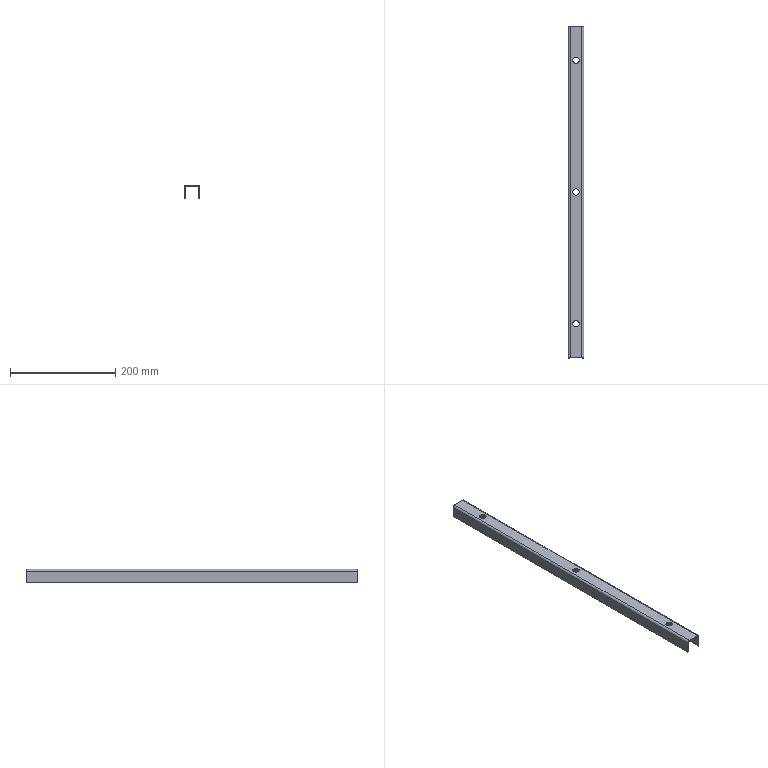Part | SolidWorks | features EdgeFlange 1, FlatPattern 1, ICE 1, SMBaseFlange 1, SheetMetal 1 | 1 solid | 28 faces | box 30 x 630 x 25 mm | volume 91837 mm3 | plane 18 | cylinder 10 | commonest cylinder face diameters 12 x6 4 x2 8 x2
STEP:
#1=CARTESIAN_POINT('',(6.,250.,-2.));
#2=VERTEX_POINT('',#1);
#3=CARTESIAN_POINT('',(-6.,250.,-2.));
#4=VERTEX_POINT('',#3);
#5=CARTESIAN_POINT('',(0.,250.,-2.));
#6=DIRECTION('',(0.,0.,-1.));
#7=DIRECTION('',(-1.,0.,0.));
#8=AXIS2_PLACEMENT_3D('',#5,#6,#7);
#9=CIRCLE('',#8,6.);
#10=EDGE_CURVE('',#2,#4,#9,.T.);
#11=ORIENTED_EDGE('',*,*,#10,.T.);
#12=CARTESIAN_POINT('',(-6.,250.,0.));
#13=VERTEX_POINT('',#12);
#14=CARTESIAN_POINT('',(-6.,250.,-25.));
#15=DIRECTION('',(0.,0.,1.));
#16=VECTOR('',#15,1000.);
#17=LINE('',#14,#16);
#18=EDGE_CURVE('',#4,#13,#17,.T.);
#19=ORIENTED_EDGE('',*,*,#18,.T.);
#20=CARTESIAN_POINT('',(6.,250.,0.));
#21=VERTEX_POINT('',#20);
#22=CARTESIAN_POINT('',(0.,250.,0.));
#23=DIRECTION('',(0.,0.,1.));
#24=DIRECTION('',(1.,0.,0.));
#25=AXIS2_PLACEMENT_3D('',#22,#23,#24);
#26=CIRCLE('',#25,6.);
#27=EDGE_CURVE('',#13,#21,#26,.T.);
#28=ORIENTED_EDGE('',*,*,#27,.T.);
#29=CARTESIAN_POINT('',(6.,250.,-25.));
#30=DIRECTION('',(0.,0.,1.));
#31=VECTOR('',#30,1000.);
#32=LINE('',#29,#31);
#33=EDGE_CURVE('',#2,#21,#32,.T.);
#34=ORIENTED_EDGE('',*,*,#33,.F.);
#35=EDGE_LOOP('',(#11,#19,#28,#34));
#36=FACE_OUTER_BOUND('',#35,.T.);
#37=CARTESIAN_POINT('',(0.,250.,-25.));
#38=DIRECTION('',(0.,0.,1.));
#39=DIRECTION('',(1.,0.,0.));
#40=AXIS2_PLACEMENT_3D('',#37,#38,#39);
#41=CYLINDRICAL_SURFACE('',#40,6.);
#42=ADVANCED_FACE('',(#36),#41,.F.);
#43=CARTESIAN_POINT('',(6.,-250.,-2.));
#44=VERTEX_POINT('',#43);
#45=CARTESIAN_POINT('',(-6.,-250.,-2.));
#46=VERTEX_POINT('',#45);
#47=CARTESIAN_POINT('',(0.,-250.,-2.));
#48=DIRECTION('',(0.,0.,-1.));
#49=DIRECTION('',(-1.,0.,0.));
#50=AXIS2_PLACEMENT_3D('',#47,#48,#49);
#51=CIRCLE('',#50,6.);
#52=EDGE_CURVE('',#44,#46,#51,.T.);
#53=ORIENTED_EDGE('',*,*,#52,.T.);
#54=CARTESIAN_POINT('',(-6.,-250.,0.));
#55=VERTEX_POINT('',#54);
#56=CARTESIAN_POINT('',(-6.,-250.,-25.));
#57=DIRECTION('',(0.,0.,1.));
#58=VECTOR('',#57,1000.);
#59=LINE('',#56,#58);
#60=EDGE_CURVE('',#46,#55,#59,.T.);
#61=ORIENTED_EDGE('',*,*,#60,.T.);
#62=CARTESIAN_POINT('',(6.,-250.,0.));
#63=VERTEX_POINT('',#62);
#64=CARTESIAN_POINT('',(0.,-250.,0.));
#65=DIRECTION('',(0.,0.,1.));
#66=DIRECTION('',(1.,0.,0.));
#67=AXIS2_PLACEMENT_3D('',#64,#65,#66);
#68=CIRCLE('',#67,6.);
#69=EDGE_CURVE('',#55,#63,#68,.T.);
#70=ORIENTED_EDGE('',*,*,#69,.T.);
#71=CARTESIAN_POINT('',(6.,-250.,-25.));
#72=DIRECTION('',(0.,0.,1.));
#73=VECTOR('',#72,1000.);
#74=LINE('',#71,#73);
#75=EDGE_CURVE('',#44,#63,#74,.T.);
#76=ORIENTED_EDGE('',*,*,#75,.F.);
#77=EDGE_LOOP('',(#53,#61,#70,#76));
#78=FACE_OUTER_BOUND('',#77,.T.);
#79=CARTESIAN_POINT('',(0.,-250.,-25.));
#80=DIRECTION('',(0.,0.,1.));
#81=DIRECTION('',(1.,0.,0.));
#82=AXIS2_PLACEMENT_3D('',#79,#80,#81);
#83=CYLINDRICAL_SURFACE('',#82,6.);
#84=ADVANCED_FACE('',(#78),#83,.F.);
#85=CARTESIAN_POINT('',(6.,0.,-2.));
#86=VERTEX_POINT('',#85);
#87=CARTESIAN_POINT('',(-6.,0.,-2.));
#88=VERTEX_POINT('',#87);
#89=CARTESIAN_POINT('',(0.,0.,-2.));
#90=DIRECTION('',(0.,0.,-1.));
#91=DIRECTION('',(-1.,0.,0.));
#92=AXIS2_PLACEMENT_3D('',#89,#90,#91);
#93=CIRCLE('',#92,6.);
#94=EDGE_CURVE('',#86,#88,#93,.T.);
#95=ORIENTED_EDGE('',*,*,#94,.T.);
#96=CARTESIAN_POINT('',(-6.,0.,0.));
#97=VERTEX_POINT('',#96);
#98=CARTESIAN_POINT('',(-6.,0.,-25.));
#99=DIRECTION('',(0.,0.,1.));
#100=VECTOR('',#99,1000.);
#101=LINE('',#98,#100);
#102=EDGE_CURVE('',#88,#97,#101,.T.);
#103=ORIENTED_EDGE('',*,*,#102,.T.);
#104=CARTESIAN_POINT('',(6.,0.,0.));
#105=VERTEX_POINT('',#104);
#106=CARTESIAN_POINT('',(0.,0.,0.));
#107=DIRECTION('',(0.,0.,1.));
#108=DIRECTION('',(1.,0.,0.));
#109=AXIS2_PLACEMENT_3D('',#106,#107,#108);
#110=CIRCLE('',#109,6.);
#111=EDGE_CURVE('',#97,#105,#110,.T.);
#112=ORIENTED_EDGE('',*,*,#111,.T.);
#113=CARTESIAN_POINT('',(6.,0.,-25.));
#114=DIRECTION('',(0.,0.,1.));
#115=VECTOR('',#114,1000.);
#116=LINE('',#113,#115);
#117=EDGE_CURVE('',#86,#105,#116,.T.);
#118=ORIENTED_EDGE('',*,*,#117,.F.);
#119=EDGE_LOOP('',(#95,#103,#112,#118));
#120=FACE_OUTER_BOUND('',#119,.T.);
#121=CARTESIAN_POINT('',(0.,0.,-25.));
#122=DIRECTION('',(0.,0.,1.));
#123=DIRECTION('',(1.,0.,0.));
#124=AXIS2_PLACEMENT_3D('',#121,#122,#123);
#125=CYLINDRICAL_SURFACE('',#124,6.);
#126=ADVANCED_FACE('',(#120),#125,.F.);
#127=ORIENTED_EDGE('',*,*,#10,.F.);
#128=CARTESIAN_POINT('',(0.,250.,-2.));
#129=DIRECTION('',(0.,0.,-1.));
#130=DIRECTION('',(-1.,0.,0.));
#131=AXIS2_PLACEMENT_3D('',#128,#129,#130);
#132=CIRCLE('',#131,6.);
#133=EDGE_CURVE('',#4,#2,#132,.T.);
#134=ORIENTED_EDGE('',*,*,#133,.F.);
#135=EDGE_LOOP('',(#127,#134));
#136=FACE_BOUND('',#135,.T.);
#137=ORIENTED_EDGE('',*,*,#52,.F.);
#138=CARTESIAN_POINT('',(0.,-250.,-2.));
#139=DIRECTION('',(0.,0.,-1.));
#140=DIRECTION('',(-1.,0.,0.));
#141=AXIS2_PLACEMENT_3D('',#138,#139,#140);
#142=CIRCLE('',#141,6.);
#143=EDGE_CURVE('',#46,#44,#142,.T.);
#144=ORIENTED_EDGE('',*,*,#143,.F.);
#145=EDGE_LOOP('',(#137,#144));
#146=FACE_BOUND('',#145,.T.);
#147=ORIENTED_EDGE('',*,*,#94,.F.);
#148=CARTESIAN_POINT('',(0.,0.,-2.));
#149=DIRECTION('',(0.,0.,-1.));
#150=DIRECTION('',(-1.,0.,0.));
#151=AXIS2_PLACEMENT_3D('',#148,#149,#150);
#152=CIRCLE('',#151,6.);
#153=EDGE_CURVE('',#88,#86,#152,.T.);
#154=ORIENTED_EDGE('',*,*,#153,.F.);
#155=EDGE_LOOP('',(#147,#154));
#156=FACE_BOUND('',#155,.T.);
#157=CARTESIAN_POINT('',(-11.,-315.,-2.));
#158=VERTEX_POINT('',#157);
#159=CARTESIAN_POINT('',(11.,-315.,-2.));
#160=VERTEX_POINT('',#159);
#161=CARTESIAN_POINT('',(-15.,-315.,-2.));
#162=DIRECTION('',(1.,0.,0.));
#163=VECTOR('',#162,1000.);
#164=LINE('',#161,#163);
#165=EDGE_CURVE('',#158,#160,#164,.T.);
#166=ORIENTED_EDGE('',*,*,#165,.F.);
#167=CARTESIAN_POINT('',(-11.,315.,-2.));
#168=VERTEX_POINT('',#167);
#169=CARTESIAN_POINT('',(-11.,315.,-2.));
#170=DIRECTION('',(0.,-1.,0.));
#171=VECTOR('',#170,1000.);
#172=LINE('',#169,#171);
#173=EDGE_CURVE('',#168,#158,#172,.T.);
#174=ORIENTED_EDGE('',*,*,#173,.F.);
#175=CARTESIAN_POINT('',(11.,315.,-2.));
#176=VERTEX_POINT('',#175);
#177=CARTESIAN_POINT('',(-15.,315.,-2.));
#178=DIRECTION('',(-1.,0.,0.));
#179=VECTOR('',#178,1000.);
#180=LINE('',#177,#179);
#181=EDGE_CURVE('',#176,#168,#180,.T.);
#182=ORIENTED_EDGE('',*,*,#181,.F.);
#183=CARTESIAN_POINT('',(11.,-315.,-2.));
#184=DIRECTION('',(0.,1.,0.));
#185=VECTOR('',#184,1000.);
#186=LINE('',#183,#185);
#187=EDGE_CURVE('',#160,#176,#186,.T.);
#188=ORIENTED_EDGE('',*,*,#187,.F.);
#189=EDGE_LOOP('',(#166,#174,#182,#188));
#190=FACE_OUTER_BOUND('',#189,.T.);
#191=CARTESIAN_POINT('',(0.,0.,-2.));
#192=DIRECTION('',(0.,0.,-1.));
#193=DIRECTION('',(-1.,0.,0.));
#194=AXIS2_PLACEMENT_3D('',#191,#192,#193);
#195=PLANE('',#194);
#196=ADVANCED_FACE('',(#136,#146,#156,#190),#195,.T.);
#197=CARTESIAN_POINT('',(0.,250.,0.));
#198=DIRECTION('',(0.,0.,1.));
#199=DIRECTION('',(1.,0.,0.));
#200=AXIS2_PLACEMENT_3D('',#197,#198,#199);
#201=CIRCLE('',#200,6.);
#202=EDGE_CURVE('',#21,#13,#201,.T.);
#203=ORIENTED_EDGE('',*,*,#202,.F.);
#204=ORIENTED_EDGE('',*,*,#27,.F.);
#205=EDGE_LOOP('',(#203,#204));
#206=FACE_BOUND('',#205,.T.);
#207=CARTESIAN_POINT('',(0.,-250.,0.));
#208=DIRECTION('',(0.,0.,1.));
#209=DIRECTION('',(1.,0.,0.));
#210=AXIS2_PLACEMENT_3D('',#207,#208,#209);
#211=CIRCLE('',#210,6.);
#212=EDGE_CURVE('',#63,#55,#211,.T.);
#213=ORIENTED_EDGE('',*,*,#212,.F.);
#214=ORIENTED_EDGE('',*,*,#69,.F.);
#215=EDGE_LOOP('',(#213,#214));
#216=FACE_BOUND('',#215,.T.);
#217=CARTESIAN_POINT('',(0.,0.,0.));
#218=DIRECTION('',(0.,0.,1.));
#219=DIRECTION('',(1.,0.,0.));
#220=AXIS2_PLACEMENT_3D('',#217,#218,#219);
#221=CIRCLE('',#220,6.);
#222=EDGE_CURVE('',#105,#97,#221,.T.);
#223=ORIENTED_EDGE('',*,*,#222,.F.);
#224=ORIENTED_EDGE('',*,*,#111,.F.);
#225=EDGE_LOOP('',(#223,#224));
#226=FACE_BOUND('',#225,.T.);
#227=CARTESIAN_POINT('',(-11.,315.,0.));
#228=VERTEX_POINT('',#227);
#229=CARTESIAN_POINT('',(-11.,-315.,0.));
#230=VERTEX_POINT('',#229);
#231=CARTESIAN_POINT('',(-11.,315.,0.));
#232=DIRECTION('',(0.,-1.,0.));
#233=VECTOR('',#232,1000.);
#234=LINE('',#231,#233);
#235=EDGE_CURVE('',#228,#230,#234,.T.);
#236=ORIENTED_EDGE('',*,*,#235,.T.);
#237=CARTESIAN_POINT('',(11.,-315.,0.));
#238=VERTEX_POINT('',#237);
#239=CARTESIAN_POINT('',(-15.,-315.,0.));
#240=DIRECTION('',(1.,0.,0.));
#241=VECTOR('',#240,1000.);
#242=LINE('',#239,#241);
#243=EDGE_CURVE('',#230,#238,#242,.T.);
#244=ORIENTED_EDGE('',*,*,#243,.T.);
#245=CARTESIAN_POINT('',(11.,315.,0.));
#246=VERTEX_POINT('',#245);
#247=CARTESIAN_POINT('',(11.,-315.,0.));
#248=DIRECTION('',(0.,1.,0.));
#249=VECTOR('',#248,1000.);
#250=LINE('',#247,#249);
#251=EDGE_CURVE('',#238,#246,#250,.T.);
#252=ORIENTED_EDGE('',*,*,#251,.T.);
#253=CARTESIAN_POINT('',(-15.,315.,0.));
#254=DIRECTION('',(-1.,0.,0.));
#255=VECTOR('',#254,1000.);
#256=LINE('',#253,#255);
#257=EDGE_CURVE('',#246,#228,#256,.T.);
#258=ORIENTED_EDGE('',*,*,#257,.T.);
#259=EDGE_LOOP('',(#236,#244,#252,#258));
#260=FACE_OUTER_BOUND('',#259,.T.);
#261=CARTESIAN_POINT('',(0.,0.,0.));
#262=DIRECTION('',(0.,0.,-1.));
#263=DIRECTION('',(-1.,0.,0.));
#264=AXIS2_PLACEMENT_3D('',#261,#262,#263);
#265=PLANE('',#264);
#266=ADVANCED_FACE('',(#206,#216,#226,#260),#265,.F.);
#267=ORIENTED_EDGE('',*,*,#181,.T.);
#268=CARTESIAN_POINT('',(-11.,315.,-2.));
#269=DIRECTION('',(0.,0.,1.));
#270=VECTOR('',#269,1000.);
#271=LINE('',#268,#270);
#272=EDGE_CURVE('',#168,#228,#271,.T.);
#273=ORIENTED_EDGE('',*,*,#272,.T.);
#274=ORIENTED_EDGE('',*,*,#257,.F.);
#275=CARTESIAN_POINT('',(11.,315.,-2.));
#276=DIRECTION('',(0.,0.,1.));
#277=VECTOR('',#276,1000.);
#278=LINE('',#275,#277);
#279=EDGE_CURVE('',#176,#246,#278,.T.);
#280=ORIENTED_EDGE('',*,*,#279,.F.);
#281=EDGE_LOOP('',(#267,#273,#274,#280));
#282=FACE_OUTER_BOUND('',#281,.T.);
#283=CARTESIAN_POINT('',(-15.,315.,-2.));
#284=DIRECTION('',(0.,1.,0.));
#285=DIRECTION('',(0.,0.,1.));
#286=AXIS2_PLACEMENT_3D('',#283,#284,#285);
#287=PLANE('',#286);
#288=ADVANCED_FACE('',(#282),#287,.T.);
#289=CARTESIAN_POINT('',(-11.,-315.,-2.));
#290=DIRECTION('',(0.,0.,1.));
#291=VECTOR('',#290,1000.);
#292=LINE('',#289,#291);
#293=EDGE_CURVE('',#158,#230,#292,.T.);
#294=ORIENTED_EDGE('',*,*,#293,.F.);
#295=ORIENTED_EDGE('',*,*,#165,.T.);
#296=CARTESIAN_POINT('',(11.,-315.,-2.));
#297=DIRECTION('',(0.,0.,1.));
#298=VECTOR('',#297,1000.);
#299=LINE('',#296,#298);
#300=EDGE_CURVE('',#160,#238,#299,.T.);
#301=ORIENTED_EDGE('',*,*,#300,.T.);
#302=ORIENTED_EDGE('',*,*,#243,.F.);
#303=EDGE_LOOP('',(#294,#295,#301,#302));
#304=FACE_OUTER_BOUND('',#303,.T.);
#305=CARTESIAN_POINT('',(-15.,-315.,-2.));
#306=DIRECTION('',(0.,-1.,0.));
#307=DIRECTION('',(0.,0.,-1.));
#308=AXIS2_PLACEMENT_3D('',#305,#306,#307);
#309=PLANE('',#308);
#310=ADVANCED_FACE('',(#304),#309,.T.);
#311=CARTESIAN_POINT('',(13.,315.,-4.));
#312=VERTEX_POINT('',#311);
#313=CARTESIAN_POINT('',(15.,315.,-4.));
#314=VERTEX_POINT('',#313);
#315=CARTESIAN_POINT('',(15.,315.,-4.));
#316=DIRECTION('',(1.,0.,0.));
#317=VECTOR('',#316,1000.);
#318=LINE('',#315,#317);
#319=EDGE_CURVE('',#312,#314,#318,.T.);
#320=ORIENTED_EDGE('',*,*,#319,.F.);
#321=CARTESIAN_POINT('',(11.,315.,-4.));
#322=DIRECTION('',(0.,1.,0.));
#323=DIRECTION('',(0.,0.,-1.));
#324=AXIS2_PLACEMENT_3D('',#321,#322,#323);
#325=CIRCLE('',#324,2.);
#326=EDGE_CURVE('',#176,#312,#325,.T.);
#327=ORIENTED_EDGE('',*,*,#326,.F.);
#328=ORIENTED_EDGE('',*,*,#279,.T.);
#329=CARTESIAN_POINT('',(11.,315.,-4.));
#330=DIRECTION('',(0.,1.,0.));
#331=DIRECTION('',(0.,0.,-1.));
#332=AXIS2_PLACEMENT_3D('',#329,#330,#331);
#333=CIRCLE('',#332,4.);
#334=EDGE_CURVE('',#246,#314,#333,.T.);
#335=ORIENTED_EDGE('',*,*,#334,.T.);
#336=EDGE_LOOP('',(#320,#327,#328,#335));
#337=FACE_OUTER_BOUND('',#336,.T.);
#338=CARTESIAN_POINT('',(11.,315.,-4.));
#339=DIRECTION('',(0.,1.,0.));
#340=DIRECTION('',(0.,0.,1.));
#341=AXIS2_PLACEMENT_3D('',#338,#339,#340);
#342=PLANE('',#341);
#343=ADVANCED_FACE('',(#337),#342,.T.);
#344=CARTESIAN_POINT('',(13.,-315.,-4.));
#345=VERTEX_POINT('',#344);
#346=CARTESIAN_POINT('',(11.,-315.,-4.));
#347=DIRECTION('',(0.,-1.,0.));
#348=DIRECTION('',(0.,0.,-1.));
#349=AXIS2_PLACEMENT_3D('',#346,#347,#348);
#350=CIRCLE('',#349,2.);
#351=EDGE_CURVE('',#345,#160,#350,.T.);
#352=ORIENTED_EDGE('',*,*,#351,.F.);
#353=CARTESIAN_POINT('',(15.,-315.,-4.));
#354=VERTEX_POINT('',#353);
#355=CARTESIAN_POINT('',(13.,-315.,-4.));
#356=DIRECTION('',(1.,0.,0.));
#357=VECTOR('',#356,1000.);
#358=LINE('',#355,#357);
#359=EDGE_CURVE('',#345,#354,#358,.T.);
#360=ORIENTED_EDGE('',*,*,#359,.T.);
#361=CARTESIAN_POINT('',(11.,-315.,-4.));
#362=DIRECTION('',(0.,-1.,0.));
#363=DIRECTION('',(0.,0.,-1.));
#364=AXIS2_PLACEMENT_3D('',#361,#362,#363);
#365=CIRCLE('',#364,4.);
#366=EDGE_CURVE('',#354,#238,#365,.T.);
#367=ORIENTED_EDGE('',*,*,#366,.T.);
#368=ORIENTED_EDGE('',*,*,#300,.F.);
#369=EDGE_LOOP('',(#352,#360,#367,#368));
#370=FACE_OUTER_BOUND('',#369,.T.);
#371=CARTESIAN_POINT('',(11.,-315.,-4.));
#372=DIRECTION('',(0.,1.,0.));
#373=DIRECTION('',(0.,0.,1.));
#374=AXIS2_PLACEMENT_3D('',#371,#372,#373);
#375=PLANE('',#374);
#376=ADVANCED_FACE('',(#370),#375,.F.);
#377=ORIENTED_EDGE('',*,*,#251,.F.);
#378=ORIENTED_EDGE('',*,*,#366,.F.);
#379=CARTESIAN_POINT('',(15.,0.,-4.));
#380=DIRECTION('',(0.,-1.,0.));
#381=VECTOR('',#380,1000.);
#382=LINE('',#379,#381);
#383=EDGE_CURVE('',#314,#354,#382,.T.);
#384=ORIENTED_EDGE('',*,*,#383,.F.);
#385=ORIENTED_EDGE('',*,*,#334,.F.);
#386=EDGE_LOOP('',(#377,#378,#384,#385));
#387=FACE_OUTER_BOUND('',#386,.T.);
#388=CARTESIAN_POINT('',(11.,-315.,-4.));
#389=DIRECTION('',(0.,-1.,0.));
#390=DIRECTION('',(1.,0.,0.));
#391=AXIS2_PLACEMENT_3D('',#388,#389,#390);
#392=CYLINDRICAL_SURFACE('',#391,4.);
#393=ADVANCED_FACE('',(#387),#392,.T.);
#394=ORIENTED_EDGE('',*,*,#187,.T.);
#395=ORIENTED_EDGE('',*,*,#326,.T.);
#396=CARTESIAN_POINT('',(13.,315.,-4.));
#397=DIRECTION('',(0.,-1.,0.));
#398=VECTOR('',#397,1000.);
#399=LINE('',#396,#398);
#400=EDGE_CURVE('',#312,#345,#399,.T.);
#401=ORIENTED_EDGE('',*,*,#400,.T.);
#402=ORIENTED_EDGE('',*,*,#351,.T.);
#403=EDGE_LOOP('',(#394,#395,#401,#402));
#404=FACE_OUTER_BOUND('',#403,.T.);
#405=CARTESIAN_POINT('',(11.,-315.,-4.));
#406=DIRECTION('',(0.,-1.,0.));
#407=DIRECTION('',(1.,0.,0.));
#408=AXIS2_PLACEMENT_3D('',#405,#406,#407);
#409=CYLINDRICAL_SURFACE('',#408,2.);
#410=ADVANCED_FACE('',(#404),#409,.F.);
#411=CARTESIAN_POINT('',(15.,-315.,-25.));
#412=VERTEX_POINT('',#411);
#413=CARTESIAN_POINT('',(15.,-315.,-2.));
#414=DIRECTION('',(0.,0.,1.));
#415=VECTOR('',#414,1000.);
#416=LINE('',#413,#415);
#417=EDGE_CURVE('',#412,#354,#416,.T.);
#418=ORIENTED_EDGE('',*,*,#417,.T.);
#419=ORIENTED_EDGE('',*,*,#359,.F.);
#420=CARTESIAN_POINT('',(13.,-315.,-25.));
#421=VERTEX_POINT('',#420);
#422=CARTESIAN_POINT('',(13.,-315.,0.));
#423=DIRECTION('',(0.,0.,1.));
#424=VECTOR('',#423,1000.);
#425=LINE('',#422,#424);
#426=EDGE_CURVE('',#421,#345,#425,.T.);
#427=ORIENTED_EDGE('',*,*,#426,.F.);
#428=CARTESIAN_POINT('',(15.,-315.,-25.));
#429=DIRECTION('',(-1.,0.,0.));
#430=VECTOR('',#429,1000.);
#431=LINE('',#428,#430);
#432=EDGE_CURVE('',#412,#421,#431,.T.);
#433=ORIENTED_EDGE('',*,*,#432,.F.);
#434=EDGE_LOOP('',(#418,#419,#427,#433));
#435=FACE_OUTER_BOUND('',#434,.T.);
#436=CARTESIAN_POINT('',(15.,-315.,-2.));
#437=DIRECTION('',(0.,-1.,0.));
#438=DIRECTION('',(0.,0.,-1.));
#439=AXIS2_PLACEMENT_3D('',#436,#437,#438);
#440=PLANE('',#439);
#441=ADVANCED_FACE('',(#435),#440,.T.);
#442=CARTESIAN_POINT('',(13.,315.,-25.));
#443=VERTEX_POINT('',#442);
#444=CARTESIAN_POINT('',(13.,315.,0.));
#445=DIRECTION('',(0.,0.,-1.));
#446=VECTOR('',#445,1000.);
#447=LINE('',#444,#446);
#448=EDGE_CURVE('',#312,#443,#447,.T.);
#449=ORIENTED_EDGE('',*,*,#448,.F.);
#450=ORIENTED_EDGE('',*,*,#319,.T.);
#451=CARTESIAN_POINT('',(15.,315.,-25.));
#452=VERTEX_POINT('',#451);
#453=CARTESIAN_POINT('',(15.,315.,-25.));
#454=DIRECTION('',(0.,0.,-1.));
#455=VECTOR('',#454,1000.);
#456=LINE('',#453,#455);
#457=EDGE_CURVE('',#314,#452,#456,.T.);
#458=ORIENTED_EDGE('',*,*,#457,.T.);
#459=CARTESIAN_POINT('',(15.,315.,-25.));
#460=DIRECTION('',(-1.,0.,0.));
#461=VECTOR('',#460,1000.);
#462=LINE('',#459,#461);
#463=EDGE_CURVE('',#452,#443,#462,.T.);
#464=ORIENTED_EDGE('',*,*,#463,.T.);
#465=EDGE_LOOP('',(#449,#450,#458,#464));
#466=FACE_OUTER_BOUND('',#465,.T.);
#467=CARTESIAN_POINT('',(15.,315.,-25.));
#468=DIRECTION('',(0.,1.,0.));
#469=DIRECTION('',(0.,0.,1.));
#470=AXIS2_PLACEMENT_3D('',#467,#468,#469);
#471=PLANE('',#470);
#472=ADVANCED_FACE('',(#466),#471,.T.);
#473=ORIENTED_EDGE('',*,*,#457,.F.);
#474=ORIENTED_EDGE('',*,*,#383,.T.);
#475=ORIENTED_EDGE('',*,*,#417,.F.);
#476=CARTESIAN_POINT('',(15.,-315.,-25.));
#477=DIRECTION('',(0.,-1.,0.));
#478=VECTOR('',#477,1000.);
#479=LINE('',#476,#478);
#480=EDGE_CURVE('',#452,#412,#479,.T.);
#481=ORIENTED_EDGE('',*,*,#480,.F.);
#482=EDGE_LOOP('',(#473,#474,#475,#481));
#483=FACE_OUTER_BOUND('',#482,.T.);
#484=CARTESIAN_POINT('',(15.,0.,0.));
#485=DIRECTION('',(1.,0.,0.));
#486=DIRECTION('',(0.,0.,-1.));
#487=AXIS2_PLACEMENT_3D('',#484,#485,#486);
#488=PLANE('',#487);
#489=ADVANCED_FACE('',(#483),#488,.T.);
#490=ORIENTED_EDGE('',*,*,#400,.F.);
#491=ORIENTED_EDGE('',*,*,#448,.T.);
#492=CARTESIAN_POINT('',(13.,0.,-25.));
#493=DIRECTION('',(0.,-1.,0.));
#494=VECTOR('',#493,1000.);
#495=LINE('',#492,#494);
#496=EDGE_CURVE('',#443,#421,#495,.T.);
#497=ORIENTED_EDGE('',*,*,#496,.T.);
#498=ORIENTED_EDGE('',*,*,#426,.T.);
#499=EDGE_LOOP('',(#490,#491,#497,#498));
#500=FACE_OUTER_BOUND('',#499,.T.);
#501=CARTESIAN_POINT('',(13.,0.,0.));
#502=DIRECTION('',(1.,0.,0.));
#503=DIRECTION('',(0.,0.,-1.));
#504=AXIS2_PLACEMENT_3D('',#501,#502,#503);
#505=PLANE('',#504);
#506=ADVANCED_FACE('',(#500),#505,.F.);
#507=ORIENTED_EDGE('',*,*,#496,.F.);
#508=ORIENTED_EDGE('',*,*,#463,.F.);
#509=ORIENTED_EDGE('',*,*,#480,.T.);
#510=ORIENTED_EDGE('',*,*,#432,.T.);
#511=EDGE_LOOP('',(#507,#508,#509,#510));
#512=FACE_OUTER_BOUND('',#511,.T.);
#513=CARTESIAN_POINT('',(15.,-315.,-25.));
#514=DIRECTION('',(0.,0.,-1.));
#515=DIRECTION('',(-1.,0.,0.));
#516=AXIS2_PLACEMENT_3D('',#513,#514,#515);
#517=PLANE('',#516);
#518=ADVANCED_FACE('',(#512),#517,.T.);
#519=CARTESIAN_POINT('',(-13.,-315.,-4.));
#520=VERTEX_POINT('',#519);
#521=CARTESIAN_POINT('',(-15.,-315.,-4.));
#522=VERTEX_POINT('',#521);
#523=CARTESIAN_POINT('',(-15.,-315.,-4.));
#524=DIRECTION('',(-1.,0.,0.));
#525=VECTOR('',#524,1000.);
#526=LINE('',#523,#525);
#527=EDGE_CURVE('',#520,#522,#526,.T.);
#528=ORIENTED_EDGE('',*,*,#527,.F.);
#529=CARTESIAN_POINT('',(-11.,-315.,-4.));
#530=DIRECTION('',(0.,-1.,0.));
#531=DIRECTION('',(0.,0.,1.));
#532=AXIS2_PLACEMENT_3D('',#529,#530,#531);
#533=CIRCLE('',#532,2.);
#534=EDGE_CURVE('',#158,#520,#533,.T.);
#535=ORIENTED_EDGE('',*,*,#534,.F.);
#536=ORIENTED_EDGE('',*,*,#293,.T.);
#537=CARTESIAN_POINT('',(-11.,-315.,-4.));
#538=DIRECTION('',(0.,-1.,0.));
#539=DIRECTION('',(0.,0.,1.));
#540=AXIS2_PLACEMENT_3D('',#537,#538,#539);
#541=CIRCLE('',#540,4.);
#542=EDGE_CURVE('',#230,#522,#541,.T.);
#543=ORIENTED_EDGE('',*,*,#542,.T.);
#544=EDGE_LOOP('',(#528,#535,#536,#543));
#545=FACE_OUTER_BOUND('',#544,.T.);
#546=CARTESIAN_POINT('',(-11.,-315.,-4.));
#547=DIRECTION('',(0.,-1.,0.));
#548=DIRECTION('',(0.,0.,-1.));
#549=AXIS2_PLACEMENT_3D('',#546,#547,#548);
#550=PLANE('',#549);
#551=ADVANCED_FACE('',(#545),#550,.T.);
#552=CARTESIAN_POINT('',(-13.,315.,-4.));
#553=VERTEX_POINT('',#552);
#554=CARTESIAN_POINT('',(-11.,315.,-4.));
#555=DIRECTION('',(0.,1.,0.));
#556=DIRECTION('',(0.,0.,1.));
#557=AXIS2_PLACEMENT_3D('',#554,#555,#556);
#558=CIRCLE('',#557,2.);
#559=EDGE_CURVE('',#553,#168,#558,.T.);
#560=ORIENTED_EDGE('',*,*,#559,.F.);
#561=CARTESIAN_POINT('',(-15.,315.,-4.));
#562=VERTEX_POINT('',#561);
#563=CARTESIAN_POINT('',(-13.,315.,-4.));
#564=DIRECTION('',(-1.,0.,0.));
#565=VECTOR('',#564,1000.);
#566=LINE('',#563,#565);
#567=EDGE_CURVE('',#553,#562,#566,.T.);
#568=ORIENTED_EDGE('',*,*,#567,.T.);
#569=CARTESIAN_POINT('',(-11.,315.,-4.));
#570=DIRECTION('',(0.,1.,0.));
#571=DIRECTION('',(0.,0.,1.));
#572=AXIS2_PLACEMENT_3D('',#569,#570,#571);
#573=CIRCLE('',#572,4.);
#574=EDGE_CURVE('',#562,#228,#573,.T.);
#575=ORIENTED_EDGE('',*,*,#574,.T.);
#576=ORIENTED_EDGE('',*,*,#272,.F.);
#577=EDGE_LOOP('',(#560,#568,#575,#576));
#578=FACE_OUTER_BOUND('',#577,.T.);
#579=CARTESIAN_POINT('',(-11.,315.,-4.));
#580=DIRECTION('',(0.,-1.,0.));
#581=DIRECTION('',(0.,0.,-1.));
#582=AXIS2_PLACEMENT_3D('',#579,#580,#581);
#583=PLANE('',#582);
#584=ADVANCED_FACE('',(#578),#583,.F.);
#585=ORIENTED_EDGE('',*,*,#235,.F.);
#586=ORIENTED_EDGE('',*,*,#574,.F.);
#587=CARTESIAN_POINT('',(-15.,-315.,-4.));
#588=DIRECTION('',(0.,-1.,0.));
#589=VECTOR('',#588,1000.);
#590=LINE('',#587,#589);
#591=EDGE_CURVE('',#562,#522,#590,.T.);
#592=ORIENTED_EDGE('',*,*,#591,.T.);
#593=ORIENTED_EDGE('',*,*,#542,.F.);
#594=EDGE_LOOP('',(#585,#586,#592,#593));
#595=FACE_OUTER_BOUND('',#594,.T.);
#596=CARTESIAN_POINT('',(-11.,315.,-4.));
#597=DIRECTION('',(0.,1.,0.));
#598=DIRECTION('',(-1.,0.,0.));
#599=AXIS2_PLACEMENT_3D('',#596,#597,#598);
#600=CYLINDRICAL_SURFACE('',#599,4.);
#601=ADVANCED_FACE('',(#595),#600,.T.);
#602=ORIENTED_EDGE('',*,*,#173,.T.);
#603=ORIENTED_EDGE('',*,*,#534,.T.);
#604=CARTESIAN_POINT('',(-13.,-315.,-4.));
#605=DIRECTION('',(0.,1.,0.));
#606=VECTOR('',#605,1000.);
#607=LINE('',#604,#606);
#608=EDGE_CURVE('',#520,#553,#607,.T.);
#609=ORIENTED_EDGE('',*,*,#608,.T.);
#610=ORIENTED_EDGE('',*,*,#559,.T.);
#611=EDGE_LOOP('',(#602,#603,#609,#610));
#612=FACE_OUTER_BOUND('',#611,.T.);
#613=CARTESIAN_POINT('',(-11.,315.,-4.));
#614=DIRECTION('',(0.,1.,0.));
#615=DIRECTION('',(-1.,0.,0.));
#616=AXIS2_PLACEMENT_3D('',#613,#614,#615);
#617=CYLINDRICAL_SURFACE('',#616,2.);
#618=ADVANCED_FACE('',(#612),#617,.F.);
#619=CARTESIAN_POINT('',(-13.,-315.,-25.));
#620=VERTEX_POINT('',#619);
#621=CARTESIAN_POINT('',(-13.,-315.,0.));
#622=DIRECTION('',(0.,0.,-1.));
#623=VECTOR('',#622,1000.);
#624=LINE('',#621,#623);
#625=EDGE_CURVE('',#520,#620,#624,.T.);
#626=ORIENTED_EDGE('',*,*,#625,.F.);
#627=ORIENTED_EDGE('',*,*,#527,.T.);
#628=CARTESIAN_POINT('',(-15.,-315.,-25.));
#629=VERTEX_POINT('',#628);
#630=CARTESIAN_POINT('',(-15.,-315.,-2.));
#631=DIRECTION('',(0.,0.,-1.));
#632=VECTOR('',#631,1000.);
#633=LINE('',#630,#632);
#634=EDGE_CURVE('',#522,#629,#633,.T.);
#635=ORIENTED_EDGE('',*,*,#634,.T.);
#636=CARTESIAN_POINT('',(-15.,-315.,-25.));
#637=DIRECTION('',(1.,0.,0.));
#638=VECTOR('',#637,1000.);
#639=LINE('',#636,#638);
#640=EDGE_CURVE('',#629,#620,#639,.T.);
#641=ORIENTED_EDGE('',*,*,#640,.T.);
#642=EDGE_LOOP('',(#626,#627,#635,#641));
#643=FACE_OUTER_BOUND('',#642,.T.);
#644=CARTESIAN_POINT('',(-15.,-315.,-2.));
#645=DIRECTION('',(0.,-1.,0.));
#646=DIRECTION('',(0.,0.,-1.));
#647=AXIS2_PLACEMENT_3D('',#644,#645,#646);
#648=PLANE('',#647);
#649=ADVANCED_FACE('',(#643),#648,.T.);
#650=CARTESIAN_POINT('',(-15.,315.,-25.));
#651=VERTEX_POINT('',#650);
#652=CARTESIAN_POINT('',(-15.,315.,-25.));
#653=DIRECTION('',(0.,0.,1.));
#654=VECTOR('',#653,1000.);
#655=LINE('',#652,#654);
#656=EDGE_CURVE('',#651,#562,#655,.T.);
#657=ORIENTED_EDGE('',*,*,#656,.T.);
#658=ORIENTED_EDGE('',*,*,#567,.F.);
#659=CARTESIAN_POINT('',(-13.,315.,-25.));
#660=VERTEX_POINT('',#659);
#661=CARTESIAN_POINT('',(-13.,315.,0.));
#662=DIRECTION('',(0.,0.,1.));
#663=VECTOR('',#662,1000.);
#664=LINE('',#661,#663);
#665=EDGE_CURVE('',#660,#553,#664,.T.);
#666=ORIENTED_EDGE('',*,*,#665,.F.);
#667=CARTESIAN_POINT('',(-15.,315.,-25.));
#668=DIRECTION('',(1.,0.,0.));
#669=VECTOR('',#668,1000.);
#670=LINE('',#667,#669);
#671=EDGE_CURVE('',#651,#660,#670,.T.);
#672=ORIENTED_EDGE('',*,*,#671,.F.);
#673=EDGE_LOOP('',(#657,#658,#666,#672));
#674=FACE_OUTER_BOUND('',#673,.T.);
#675=CARTESIAN_POINT('',(-15.,315.,-25.));
#676=DIRECTION('',(0.,1.,0.));
#677=DIRECTION('',(0.,0.,1.));
#678=AXIS2_PLACEMENT_3D('',#675,#676,#677);
#679=PLANE('',#678);
#680=ADVANCED_FACE('',(#674),#679,.T.);
#681=ORIENTED_EDGE('',*,*,#591,.F.);
#682=ORIENTED_EDGE('',*,*,#656,.F.);
#683=CARTESIAN_POINT('',(-15.,-315.,-25.));
#684=DIRECTION('',(0.,1.,0.));
#685=VECTOR('',#684,1000.);
#686=LINE('',#683,#685);
#687=EDGE_CURVE('',#629,#651,#686,.T.);
#688=ORIENTED_EDGE('',*,*,#687,.F.);
#689=ORIENTED_EDGE('',*,*,#634,.F.);
#690=EDGE_LOOP('',(#681,#682,#688,#689));
#691=FACE_OUTER_BOUND('',#690,.T.);
#692=CARTESIAN_POINT('',(-15.,0.,0.));
#693=DIRECTION('',(1.,0.,0.));
#694=DIRECTION('',(0.,0.,-1.));
#695=AXIS2_PLACEMENT_3D('',#692,#693,#694);
#696=PLANE('',#695);
#697=ADVANCED_FACE('',(#691),#696,.F.);
#698=ORIENTED_EDGE('',*,*,#665,.T.);
#699=ORIENTED_EDGE('',*,*,#608,.F.);
#700=ORIENTED_EDGE('',*,*,#625,.T.);
#701=CARTESIAN_POINT('',(-13.,0.,-25.));
#702=DIRECTION('',(0.,1.,0.));
#703=VECTOR('',#702,1000.);
#704=LINE('',#701,#703);
#705=EDGE_CURVE('',#620,#660,#704,.T.);
#706=ORIENTED_EDGE('',*,*,#705,.T.);
#707=EDGE_LOOP('',(#698,#699,#700,#706));
#708=FACE_OUTER_BOUND('',#707,.T.);
#709=CARTESIAN_POINT('',(-13.,0.,0.));
#710=DIRECTION('',(1.,0.,0.));
#711=DIRECTION('',(0.,0.,-1.));
#712=AXIS2_PLACEMENT_3D('',#709,#710,#711);
#713=PLANE('',#712);
#714=ADVANCED_FACE('',(#708),#713,.T.);
#715=ORIENTED_EDGE('',*,*,#705,.F.);
#716=ORIENTED_EDGE('',*,*,#640,.F.);
#717=ORIENTED_EDGE('',*,*,#687,.T.);
#718=ORIENTED_EDGE('',*,*,#671,.T.);
#719=EDGE_LOOP('',(#715,#716,#717,#718));
#720=FACE_OUTER_BOUND('',#719,.T.);
#721=CARTESIAN_POINT('',(-15.,-315.,-25.));
#722=DIRECTION('',(0.,0.,-1.));
#723=DIRECTION('',(-1.,0.,0.));
#724=AXIS2_PLACEMENT_3D('',#721,#722,#723);
#725=PLANE('',#724);
#726=ADVANCED_FACE('',(#720),#725,.T.);
#727=ORIENTED_EDGE('',*,*,#102,.F.);
#728=ORIENTED_EDGE('',*,*,#153,.T.);
#729=ORIENTED_EDGE('',*,*,#117,.T.);
#730=ORIENTED_EDGE('',*,*,#222,.T.);
#731=EDGE_LOOP('',(#727,#728,#729,#730));
#732=FACE_OUTER_BOUND('',#731,.T.);
#733=CARTESIAN_POINT('',(0.,0.,-25.));
#734=DIRECTION('',(0.,0.,1.));
#735=DIRECTION('',(1.,0.,0.));
#736=AXIS2_PLACEMENT_3D('',#733,#734,#735);
#737=CYLINDRICAL_SURFACE('',#736,6.);
#738=ADVANCED_FACE('',(#732),#737,.F.);
#739=ORIENTED_EDGE('',*,*,#60,.F.);
#740=ORIENTED_EDGE('',*,*,#143,.T.);
#741=ORIENTED_EDGE('',*,*,#75,.T.);
#742=ORIENTED_EDGE('',*,*,#212,.T.);
#743=EDGE_LOOP('',(#739,#740,#741,#742));
#744=FACE_OUTER_BOUND('',#743,.T.);
#745=CARTESIAN_POINT('',(0.,-250.,-25.));
#746=DIRECTION('',(0.,0.,1.));
#747=DIRECTION('',(1.,0.,0.));
#748=AXIS2_PLACEMENT_3D('',#745,#746,#747);
#749=CYLINDRICAL_SURFACE('',#748,6.);
#750=ADVANCED_FACE('',(#744),#749,.F.);
#751=ORIENTED_EDGE('',*,*,#18,.F.);
#752=ORIENTED_EDGE('',*,*,#133,.T.);
#753=ORIENTED_EDGE('',*,*,#33,.T.);
#754=ORIENTED_EDGE('',*,*,#202,.T.);
#755=EDGE_LOOP('',(#751,#752,#753,#754));
#756=FACE_OUTER_BOUND('',#755,.T.);
#757=CARTESIAN_POINT('',(0.,250.,-25.));
#758=DIRECTION('',(0.,0.,1.));
#759=DIRECTION('',(1.,0.,0.));
#760=AXIS2_PLACEMENT_3D('',#757,#758,#759);
#761=CYLINDRICAL_SURFACE('',#760,6.);
#762=ADVANCED_FACE('',(#756),#761,.F.);
#763=CLOSED_SHELL('',(#42,#84,#126,#196,#266,#288,#310,#343,#376,#393,#410,#441,#472,#489,#506,#518,#551,#584,#601,#618,#649,#680,#697,#714,#726,#738,#750,#762));
#764=MANIFOLD_SOLID_BREP('',#763);
#765=CARTESIAN_POINT('',(0.,0.,0.));
#766=DIRECTION('',(0.,0.,1.));
#767=DIRECTION('',(1.,0.,0.));
#768=AXIS2_PLACEMENT_3D('',#765,#766,#767);
#769=(LENGTH_UNIT()NAMED_UNIT(*)SI_UNIT(.MILLI.,.METRE.));
#770=UNCERTAINTY_MEASURE_WITH_UNIT(LENGTH_MEASURE(0.00001),#769,'','');
#771=(NAMED_UNIT(*)PLANE_ANGLE_UNIT()SI_UNIT($,.RADIAN.));
#772=(NAMED_UNIT(*)SI_UNIT($,.STERADIAN.)SOLID_ANGLE_UNIT());
#773=(GEOMETRIC_REPRESENTATION_CONTEXT(3)GLOBAL_UNCERTAINTY_ASSIGNED_CONTEXT((#770))GLOBAL_UNIT_ASSIGNED_CONTEXT((#769,#771,#772))REPRESENTATION_CONTEXT('',''));
#774=ADVANCED_BREP_SHAPE_REPRESENTATION('',(#764,#768),#773);